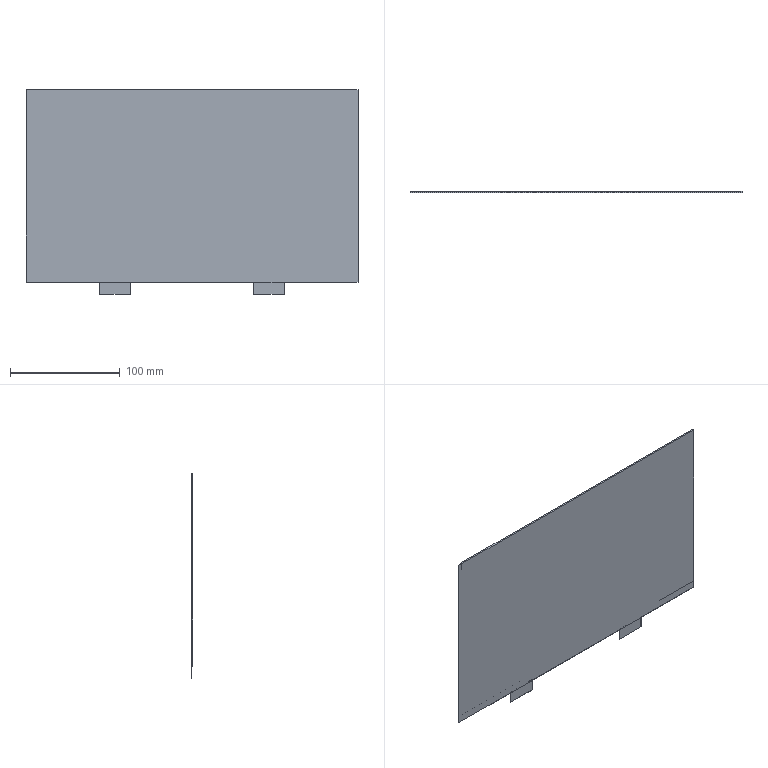Part | SolidWorks | features ICE 4, Extrusion 1, LPattern 1 | 1 solid | 56 faces | box 301.97 x 1.43 x 186.39 mm | volume 73825 mm3 | plane 42 | spline 14